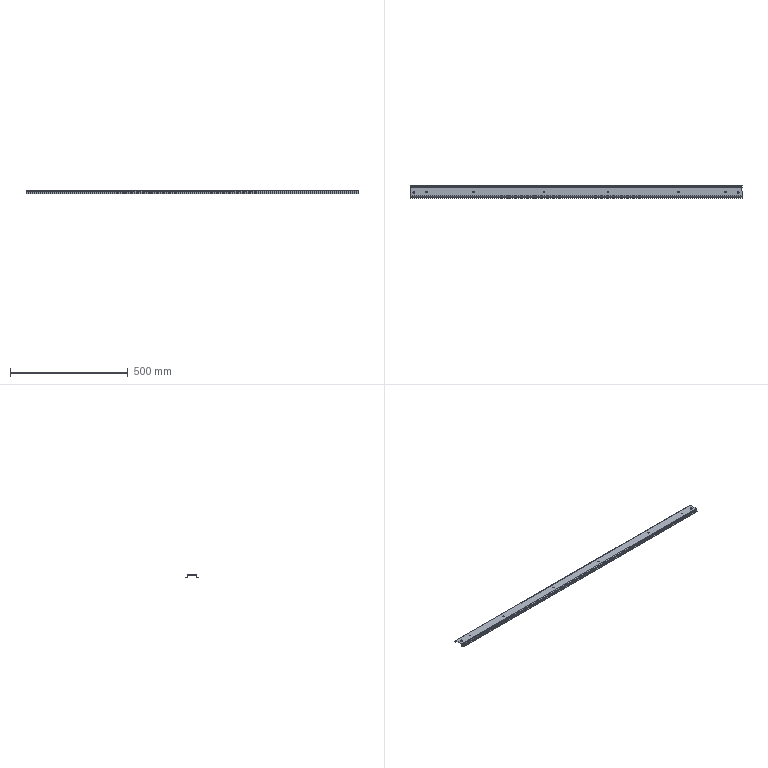Part | SolidWorks | features EdgeFlange 2, MirrorPattern 2, 3DProfileFeature 1, Cut 1, FlatPattern 1, HoleWzd 1, ICE 1, SMBaseFlange 1, SheetMetal 1 | 1 solid | 60 faces | box 1410 x 53 x 13 mm | volume 143996 mm3 | plane 32 | cylinder 28 | commonest cylinder face diameters 6 x16 3 x4 4.2 x4 8.7 x4